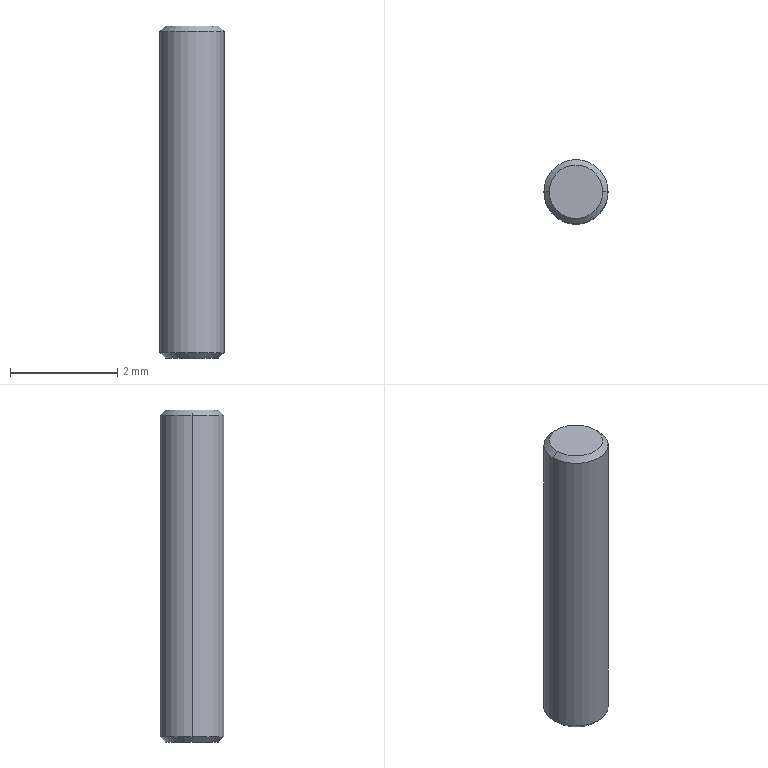Part | SolidWorks | features Chamfer 1, Extrusion 1 | 1 solid | 8 faces | box 1.2 x 1.2 x 6.2 mm | volume 6.976 mm3 | cone 4 | cylinder 2 | plane 2 | commonest cylinder face diameters 1.2 x2
STEP:
#1=CARTESIAN_POINT('',(0.5,0.,3.1));
#2=VERTEX_POINT('',#1);
#3=CARTESIAN_POINT('',(-0.5,0.,3.1));
#4=VERTEX_POINT('',#3);
#5=CARTESIAN_POINT('',(0.,0.,3.1));
#6=DIRECTION('',(0.,0.,1.));
#7=DIRECTION('',(1.,0.,0.));
#8=AXIS2_PLACEMENT_3D('',#5,#6,#7);
#9=CIRCLE('',#8,0.5);
#10=EDGE_CURVE('',#2,#4,#9,.T.);
#11=ORIENTED_EDGE('',*,*,#10,.F.);
#12=CARTESIAN_POINT('',(0.6,0.,3.));
#13=VERTEX_POINT('',#12);
#14=CARTESIAN_POINT('',(0.5,0.,3.1));
#15=DIRECTION('',(0.7071,0.,-0.7071));
#16=VECTOR('',#15,1000.);
#17=LINE('',#14,#16);
#18=EDGE_CURVE('',#2,#13,#17,.T.);
#19=ORIENTED_EDGE('',*,*,#18,.T.);
#20=CARTESIAN_POINT('',(-0.6,0.,3.));
#21=VERTEX_POINT('',#20);
#22=CARTESIAN_POINT('',(0.,0.,3.));
#23=DIRECTION('',(0.,0.,-1.));
#24=DIRECTION('',(1.,0.,0.));
#25=AXIS2_PLACEMENT_3D('',#22,#23,#24);
#26=CIRCLE('',#25,0.6);
#27=EDGE_CURVE('',#21,#13,#26,.T.);
#28=ORIENTED_EDGE('',*,*,#27,.F.);
#29=CARTESIAN_POINT('',(-0.5,0.,3.1));
#30=DIRECTION('',(-0.7071,0.,-0.7071));
#31=VECTOR('',#30,1000.);
#32=LINE('',#29,#31);
#33=EDGE_CURVE('',#4,#21,#32,.T.);
#34=ORIENTED_EDGE('',*,*,#33,.F.);
#35=EDGE_LOOP('',(#11,#19,#28,#34));
#36=FACE_OUTER_BOUND('',#35,.T.);
#37=CARTESIAN_POINT('',(0.,0.,3.1));
#38=DIRECTION('',(0.,0.,-1.));
#39=DIRECTION('',(-1.,0.,0.));
#40=AXIS2_PLACEMENT_3D('',#37,#38,#39);
#41=CONICAL_SURFACE('',#40,0.5,0.7854);
#42=ADVANCED_FACE('',(#36),#41,.T.);
#43=CARTESIAN_POINT('',(-0.5,0.,-3.1));
#44=VERTEX_POINT('',#43);
#45=CARTESIAN_POINT('',(0.5,0.,-3.1));
#46=VERTEX_POINT('',#45);
#47=CARTESIAN_POINT('',(0.,0.,-3.1));
#48=DIRECTION('',(0.,0.,-1.));
#49=DIRECTION('',(1.,0.,0.));
#50=AXIS2_PLACEMENT_3D('',#47,#48,#49);
#51=CIRCLE('',#50,0.5);
#52=EDGE_CURVE('',#44,#46,#51,.T.);
#53=ORIENTED_EDGE('',*,*,#52,.F.);
#54=CARTESIAN_POINT('',(-0.6,0.,-3.));
#55=VERTEX_POINT('',#54);
#56=CARTESIAN_POINT('',(-0.6,0.,-3.));
#57=DIRECTION('',(-0.7071,0.,0.7071));
#58=VECTOR('',#57,1000.);
#59=LINE('',#56,#58);
#60=EDGE_CURVE('',#44,#55,#59,.T.);
#61=ORIENTED_EDGE('',*,*,#60,.T.);
#62=CARTESIAN_POINT('',(0.6,0.,-3.));
#63=VERTEX_POINT('',#62);
#64=CARTESIAN_POINT('',(0.,0.,-3.));
#65=DIRECTION('',(0.,0.,1.));
#66=DIRECTION('',(1.,0.,0.));
#67=AXIS2_PLACEMENT_3D('',#64,#65,#66);
#68=CIRCLE('',#67,0.6);
#69=EDGE_CURVE('',#63,#55,#68,.T.);
#70=ORIENTED_EDGE('',*,*,#69,.F.);
#71=CARTESIAN_POINT('',(0.6,0.,-3.));
#72=DIRECTION('',(0.7071,0.,0.7071));
#73=VECTOR('',#72,1000.);
#74=LINE('',#71,#73);
#75=EDGE_CURVE('',#46,#63,#74,.T.);
#76=ORIENTED_EDGE('',*,*,#75,.F.);
#77=EDGE_LOOP('',(#53,#61,#70,#76));
#78=FACE_OUTER_BOUND('',#77,.T.);
#79=CARTESIAN_POINT('',(0.,0.,-3.));
#80=DIRECTION('',(0.,0.,1.));
#81=DIRECTION('',(1.,0.,0.));
#82=AXIS2_PLACEMENT_3D('',#79,#80,#81);
#83=CONICAL_SURFACE('',#82,0.6,0.7854);
#84=ADVANCED_FACE('',(#78),#83,.T.);
#85=ORIENTED_EDGE('',*,*,#27,.T.);
#86=CARTESIAN_POINT('',(0.6,0.,3.1));
#87=DIRECTION('',(0.,0.,-1.));
#88=VECTOR('',#87,1000.);
#89=LINE('',#86,#88);
#90=EDGE_CURVE('',#13,#63,#89,.T.);
#91=ORIENTED_EDGE('',*,*,#90,.T.);
#92=ORIENTED_EDGE('',*,*,#69,.T.);
#93=CARTESIAN_POINT('',(-0.6,0.,3.1));
#94=DIRECTION('',(0.,0.,-1.));
#95=VECTOR('',#94,1000.);
#96=LINE('',#93,#95);
#97=EDGE_CURVE('',#21,#55,#96,.T.);
#98=ORIENTED_EDGE('',*,*,#97,.F.);
#99=EDGE_LOOP('',(#85,#91,#92,#98));
#100=FACE_OUTER_BOUND('',#99,.T.);
#101=CARTESIAN_POINT('',(0.,0.,3.1));
#102=DIRECTION('',(0.,0.,-1.));
#103=DIRECTION('',(-1.,0.,0.));
#104=AXIS2_PLACEMENT_3D('',#101,#102,#103);
#105=CYLINDRICAL_SURFACE('',#104,0.6);
#106=ADVANCED_FACE('',(#100),#105,.T.);
#107=ORIENTED_EDGE('',*,*,#90,.F.);
#108=CARTESIAN_POINT('',(0.,0.,3.));
#109=DIRECTION('',(0.,0.,-1.));
#110=DIRECTION('',(1.,0.,0.));
#111=AXIS2_PLACEMENT_3D('',#108,#109,#110);
#112=CIRCLE('',#111,0.6);
#113=EDGE_CURVE('',#13,#21,#112,.T.);
#114=ORIENTED_EDGE('',*,*,#113,.T.);
#115=ORIENTED_EDGE('',*,*,#97,.T.);
#116=CARTESIAN_POINT('',(0.,0.,-3.));
#117=DIRECTION('',(0.,0.,1.));
#118=DIRECTION('',(1.,0.,0.));
#119=AXIS2_PLACEMENT_3D('',#116,#117,#118);
#120=CIRCLE('',#119,0.6);
#121=EDGE_CURVE('',#55,#63,#120,.T.);
#122=ORIENTED_EDGE('',*,*,#121,.T.);
#123=EDGE_LOOP('',(#107,#114,#115,#122));
#124=FACE_OUTER_BOUND('',#123,.T.);
#125=CARTESIAN_POINT('',(0.,0.,3.1));
#126=DIRECTION('',(0.,0.,-1.));
#127=DIRECTION('',(-1.,0.,0.));
#128=AXIS2_PLACEMENT_3D('',#125,#126,#127);
#129=CYLINDRICAL_SURFACE('',#128,0.6);
#130=ADVANCED_FACE('',(#124),#129,.T.);
#131=CARTESIAN_POINT('',(0.,0.,3.1));
#132=DIRECTION('',(0.,0.,1.));
#133=DIRECTION('',(1.,0.,0.));
#134=AXIS2_PLACEMENT_3D('',#131,#132,#133);
#135=CIRCLE('',#134,0.5);
#136=EDGE_CURVE('',#4,#2,#135,.T.);
#137=ORIENTED_EDGE('',*,*,#136,.T.);
#138=ORIENTED_EDGE('',*,*,#10,.T.);
#139=EDGE_LOOP('',(#137,#138));
#140=FACE_OUTER_BOUND('',#139,.T.);
#141=CARTESIAN_POINT('',(0.,0.,3.1));
#142=DIRECTION('',(0.,0.,1.));
#143=DIRECTION('',(1.,0.,0.));
#144=AXIS2_PLACEMENT_3D('',#141,#142,#143);
#145=PLANE('',#144);
#146=ADVANCED_FACE('',(#140),#145,.T.);
#147=CARTESIAN_POINT('',(0.,0.,-3.1));
#148=DIRECTION('',(0.,0.,-1.));
#149=DIRECTION('',(1.,0.,0.));
#150=AXIS2_PLACEMENT_3D('',#147,#148,#149);
#151=CIRCLE('',#150,0.5);
#152=EDGE_CURVE('',#46,#44,#151,.T.);
#153=ORIENTED_EDGE('',*,*,#152,.T.);
#154=ORIENTED_EDGE('',*,*,#52,.T.);
#155=EDGE_LOOP('',(#153,#154));
#156=FACE_OUTER_BOUND('',#155,.T.);
#157=CARTESIAN_POINT('',(0.,0.,-3.1));
#158=DIRECTION('',(0.,0.,1.));
#159=DIRECTION('',(1.,0.,0.));
#160=AXIS2_PLACEMENT_3D('',#157,#158,#159);
#161=PLANE('',#160);
#162=ADVANCED_FACE('',(#156),#161,.F.);
#163=ORIENTED_EDGE('',*,*,#60,.F.);
#164=ORIENTED_EDGE('',*,*,#152,.F.);
#165=ORIENTED_EDGE('',*,*,#75,.T.);
#166=ORIENTED_EDGE('',*,*,#121,.F.);
#167=EDGE_LOOP('',(#163,#164,#165,#166));
#168=FACE_OUTER_BOUND('',#167,.T.);
#169=CARTESIAN_POINT('',(0.,0.,-3.));
#170=DIRECTION('',(0.,0.,1.));
#171=DIRECTION('',(1.,0.,0.));
#172=AXIS2_PLACEMENT_3D('',#169,#170,#171);
#173=CONICAL_SURFACE('',#172,0.6,0.7854);
#174=ADVANCED_FACE('',(#168),#173,.T.);
#175=ORIENTED_EDGE('',*,*,#18,.F.);
#176=ORIENTED_EDGE('',*,*,#136,.F.);
#177=ORIENTED_EDGE('',*,*,#33,.T.);
#178=ORIENTED_EDGE('',*,*,#113,.F.);
#179=EDGE_LOOP('',(#175,#176,#177,#178));
#180=FACE_OUTER_BOUND('',#179,.T.);
#181=CARTESIAN_POINT('',(0.,0.,3.1));
#182=DIRECTION('',(0.,0.,-1.));
#183=DIRECTION('',(-1.,0.,0.));
#184=AXIS2_PLACEMENT_3D('',#181,#182,#183);
#185=CONICAL_SURFACE('',#184,0.5,0.7854);
#186=ADVANCED_FACE('',(#180),#185,.T.);
#187=CLOSED_SHELL('',(#42,#84,#106,#130,#146,#162,#174,#186));
#188=MANIFOLD_SOLID_BREP('',#187);
#189=CARTESIAN_POINT('',(0.,0.,0.));
#190=DIRECTION('',(0.,0.,1.));
#191=DIRECTION('',(1.,0.,0.));
#192=AXIS2_PLACEMENT_3D('',#189,#190,#191);
#193=(LENGTH_UNIT()NAMED_UNIT(*)SI_UNIT(.MILLI.,.METRE.));
#194=UNCERTAINTY_MEASURE_WITH_UNIT(LENGTH_MEASURE(0.00001),#193,'','');
#195=(NAMED_UNIT(*)PLANE_ANGLE_UNIT()SI_UNIT($,.RADIAN.));
#196=(NAMED_UNIT(*)SI_UNIT($,.STERADIAN.)SOLID_ANGLE_UNIT());
#197=(GEOMETRIC_REPRESENTATION_CONTEXT(3)GLOBAL_UNCERTAINTY_ASSIGNED_CONTEXT((#194))GLOBAL_UNIT_ASSIGNED_CONTEXT((#193,#195,#196))REPRESENTATION_CONTEXT('',''));
#198=ADVANCED_BREP_SHAPE_REPRESENTATION('',(#188,#192),#197);